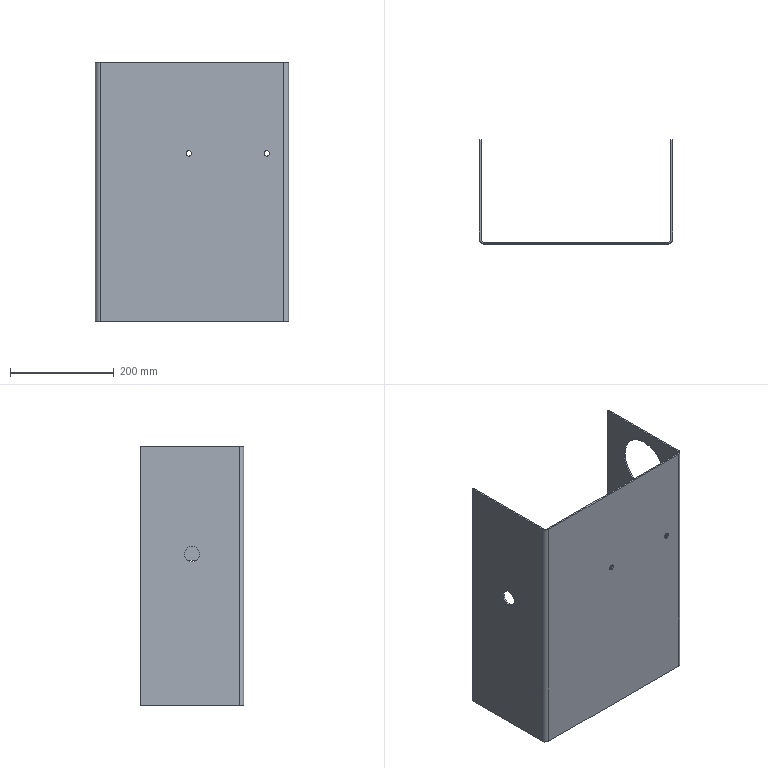Part | SolidWorks | features Cut 4, FlatPattern 1, SMBaseFlange 1, SheetMetal 1 | 1 solid | 34 faces | box 372 x 200 x 500 mm | volume 1068373 mm3 | plane 18 | cylinder 16 | commonest cylinder face diameters 10.5 x4 12 x2 18 x2 30 x2 50 x2 110 x2
STEP:
#1=CARTESIAN_POINT('',(-638.867,1083.196,324.485));
#2=VERTEX_POINT('',#1);
#3=CARTESIAN_POINT('',(-628.367,1083.196,324.485));
#4=VERTEX_POINT('',#3);
#5=CARTESIAN_POINT('',(-633.617,1083.196,324.485));
#6=DIRECTION('',(0.,-1.,0.));
#7=DIRECTION('',(1.,0.,0.));
#8=AXIS2_PLACEMENT_3D('',#5,#6,#7);
#9=CIRCLE('',#8,5.25);
#10=EDGE_CURVE('',#2,#4,#9,.T.);
#11=ORIENTED_EDGE('',*,*,#10,.F.);
#12=CARTESIAN_POINT('',(-638.867,1080.196,324.485));
#13=VERTEX_POINT('',#12);
#14=CARTESIAN_POINT('',(-638.867,1090.196,324.485));
#15=DIRECTION('',(0.,-1.,0.));
#16=VECTOR('',#15,1000.);
#17=LINE('',#14,#16);
#18=EDGE_CURVE('',#2,#13,#17,.T.);
#19=ORIENTED_EDGE('',*,*,#18,.T.);
#20=CARTESIAN_POINT('',(-628.367,1080.196,324.485));
#21=VERTEX_POINT('',#20);
#22=CARTESIAN_POINT('',(-633.617,1080.196,324.485));
#23=DIRECTION('',(0.,-1.,0.));
#24=DIRECTION('',(1.,0.,0.));
#25=AXIS2_PLACEMENT_3D('',#22,#23,#24);
#26=CIRCLE('',#25,5.25);
#27=EDGE_CURVE('',#13,#21,#26,.T.);
#28=ORIENTED_EDGE('',*,*,#27,.T.);
#29=CARTESIAN_POINT('',(-628.367,1090.196,324.485));
#30=DIRECTION('',(0.,-1.,0.));
#31=VECTOR('',#30,1000.);
#32=LINE('',#29,#31);
#33=EDGE_CURVE('',#4,#21,#32,.T.);
#34=ORIENTED_EDGE('',*,*,#33,.F.);
#35=EDGE_LOOP('',(#11,#19,#28,#34));
#36=FACE_OUTER_BOUND('',#35,.T.);
#37=CARTESIAN_POINT('',(-633.617,1090.196,324.485));
#38=DIRECTION('',(0.,-1.,0.));
#39=DIRECTION('',(1.,0.,0.));
#40=AXIS2_PLACEMENT_3D('',#37,#38,#39);
#41=CYLINDRICAL_SURFACE('',#40,5.25);
#42=ADVANCED_FACE('',(#36),#41,.F.);
#43=CARTESIAN_POINT('',(-788.867,1083.196,324.485));
#44=VERTEX_POINT('',#43);
#45=CARTESIAN_POINT('',(-778.367,1083.196,324.485));
#46=VERTEX_POINT('',#45);
#47=CARTESIAN_POINT('',(-783.617,1083.196,324.485));
#48=DIRECTION('',(0.,-1.,0.));
#49=DIRECTION('',(1.,0.,0.));
#50=AXIS2_PLACEMENT_3D('',#47,#48,#49);
#51=CIRCLE('',#50,5.25);
#52=EDGE_CURVE('',#44,#46,#51,.T.);
#53=ORIENTED_EDGE('',*,*,#52,.F.);
#54=CARTESIAN_POINT('',(-788.867,1080.196,324.485));
#55=VERTEX_POINT('',#54);
#56=CARTESIAN_POINT('',(-788.867,1090.196,324.485));
#57=DIRECTION('',(0.,-1.,0.));
#58=VECTOR('',#57,1000.);
#59=LINE('',#56,#58);
#60=EDGE_CURVE('',#44,#55,#59,.T.);
#61=ORIENTED_EDGE('',*,*,#60,.T.);
#62=CARTESIAN_POINT('',(-778.367,1080.196,324.485));
#63=VERTEX_POINT('',#62);
#64=CARTESIAN_POINT('',(-783.617,1080.196,324.485));
#65=DIRECTION('',(0.,-1.,0.));
#66=DIRECTION('',(1.,0.,0.));
#67=AXIS2_PLACEMENT_3D('',#64,#65,#66);
#68=CIRCLE('',#67,5.25);
#69=EDGE_CURVE('',#55,#63,#68,.T.);
#70=ORIENTED_EDGE('',*,*,#69,.T.);
#71=CARTESIAN_POINT('',(-778.367,1090.196,324.485));
#72=DIRECTION('',(0.,-1.,0.));
#73=VECTOR('',#72,1000.);
#74=LINE('',#71,#73);
#75=EDGE_CURVE('',#46,#63,#74,.T.);
#76=ORIENTED_EDGE('',*,*,#75,.F.);
#77=EDGE_LOOP('',(#53,#61,#70,#76));
#78=FACE_OUTER_BOUND('',#77,.T.);
#79=CARTESIAN_POINT('',(-783.617,1090.196,324.485));
#80=DIRECTION('',(0.,-1.,0.));
#81=DIRECTION('',(1.,0.,0.));
#82=AXIS2_PLACEMENT_3D('',#79,#80,#81);
#83=CYLINDRICAL_SURFACE('',#82,5.25);
#84=ADVANCED_FACE('',(#78),#83,.F.);
#85=CARTESIAN_POINT('',(-960.617,1195.196,292.));
#86=VERTEX_POINT('',#85);
#87=CARTESIAN_POINT('',(-960.617,1165.196,292.));
#88=VERTEX_POINT('',#87);
#89=CARTESIAN_POINT('',(-960.617,1180.196,292.));
#90=DIRECTION('',(-1.,0.,0.));
#91=DIRECTION('',(0.,-1.,0.));
#92=AXIS2_PLACEMENT_3D('',#89,#90,#91);
#93=CIRCLE('',#92,15.);
#94=EDGE_CURVE('',#86,#88,#93,.T.);
#95=ORIENTED_EDGE('',*,*,#94,.F.);
#96=CARTESIAN_POINT('',(-963.617,1195.196,292.));
#97=VERTEX_POINT('',#96);
#98=CARTESIAN_POINT('',(-953.617,1195.196,292.));
#99=DIRECTION('',(-1.,0.,0.));
#100=VECTOR('',#99,1000.);
#101=LINE('',#98,#100);
#102=EDGE_CURVE('',#86,#97,#101,.T.);
#103=ORIENTED_EDGE('',*,*,#102,.T.);
#104=CARTESIAN_POINT('',(-963.617,1165.196,292.));
#105=VERTEX_POINT('',#104);
#106=CARTESIAN_POINT('',(-963.617,1180.196,292.));
#107=DIRECTION('',(-1.,0.,0.));
#108=DIRECTION('',(0.,-1.,0.));
#109=AXIS2_PLACEMENT_3D('',#106,#107,#108);
#110=CIRCLE('',#109,15.);
#111=EDGE_CURVE('',#97,#105,#110,.T.);
#112=ORIENTED_EDGE('',*,*,#111,.T.);
#113=CARTESIAN_POINT('',(-953.617,1165.196,292.));
#114=DIRECTION('',(-1.,0.,0.));
#115=VECTOR('',#114,1000.);
#116=LINE('',#113,#115);
#117=EDGE_CURVE('',#88,#105,#116,.T.);
#118=ORIENTED_EDGE('',*,*,#117,.F.);
#119=EDGE_LOOP('',(#95,#103,#112,#118));
#120=FACE_OUTER_BOUND('',#119,.T.);
#121=CARTESIAN_POINT('',(-953.617,1180.196,292.));
#122=DIRECTION('',(-1.,0.,0.));
#123=DIRECTION('',(0.,-1.,0.));
#124=AXIS2_PLACEMENT_3D('',#121,#122,#123);
#125=CYLINDRICAL_SURFACE('',#124,15.);
#126=ADVANCED_FACE('',(#120),#125,.F.);
#127=CARTESIAN_POINT('',(-594.617,1137.696,95.));
#128=VERTEX_POINT('',#127);
#129=CARTESIAN_POINT('',(-594.617,1137.696,45.));
#130=VERTEX_POINT('',#129);
#131=CARTESIAN_POINT('',(-594.617,1137.696,70.));
#132=DIRECTION('',(1.,0.,0.));
#133=DIRECTION('',(0.,0.,-1.));
#134=AXIS2_PLACEMENT_3D('',#131,#132,#133);
#135=CIRCLE('',#134,25.);
#136=EDGE_CURVE('',#128,#130,#135,.T.);
#137=ORIENTED_EDGE('',*,*,#136,.F.);
#138=CARTESIAN_POINT('',(-591.617,1137.696,95.));
#139=VERTEX_POINT('',#138);
#140=CARTESIAN_POINT('',(-601.617,1137.696,95.));
#141=DIRECTION('',(1.,0.,0.));
#142=VECTOR('',#141,1000.);
#143=LINE('',#140,#142);
#144=EDGE_CURVE('',#128,#139,#143,.T.);
#145=ORIENTED_EDGE('',*,*,#144,.T.);
#146=CARTESIAN_POINT('',(-591.617,1137.696,45.));
#147=VERTEX_POINT('',#146);
#148=CARTESIAN_POINT('',(-591.617,1137.696,70.));
#149=DIRECTION('',(1.,0.,0.));
#150=DIRECTION('',(0.,0.,-1.));
#151=AXIS2_PLACEMENT_3D('',#148,#149,#150);
#152=CIRCLE('',#151,25.);
#153=EDGE_CURVE('',#139,#147,#152,.T.);
#154=ORIENTED_EDGE('',*,*,#153,.T.);
#155=CARTESIAN_POINT('',(-601.617,1137.696,45.));
#156=DIRECTION('',(1.,0.,0.));
#157=VECTOR('',#156,1000.);
#158=LINE('',#155,#157);
#159=EDGE_CURVE('',#130,#147,#158,.T.);
#160=ORIENTED_EDGE('',*,*,#159,.F.);
#161=EDGE_LOOP('',(#137,#145,#154,#160));
#162=FACE_OUTER_BOUND('',#161,.T.);
#163=CARTESIAN_POINT('',(-601.617,1137.696,70.));
#164=DIRECTION('',(1.,0.,0.));
#165=DIRECTION('',(0.,0.,-1.));
#166=AXIS2_PLACEMENT_3D('',#163,#164,#165);
#167=CYLINDRICAL_SURFACE('',#166,25.);
#168=ADVANCED_FACE('',(#162),#167,.F.);
#169=CARTESIAN_POINT('',(-594.617,1180.196,280.));
#170=VERTEX_POINT('',#169);
#171=CARTESIAN_POINT('',(-594.617,1180.196,160.));
#172=VERTEX_POINT('',#171);
#173=CARTESIAN_POINT('',(-594.617,1180.196,220.));
#174=DIRECTION('',(1.,0.,0.));
#175=DIRECTION('',(0.,0.,-1.));
#176=AXIS2_PLACEMENT_3D('',#173,#174,#175);
#177=CIRCLE('',#176,60.);
#178=EDGE_CURVE('',#170,#172,#177,.T.);
#179=ORIENTED_EDGE('',*,*,#178,.F.);
#180=CARTESIAN_POINT('',(-591.617,1180.196,280.));
#181=VERTEX_POINT('',#180);
#182=CARTESIAN_POINT('',(-601.617,1180.196,280.));
#183=DIRECTION('',(1.,0.,0.));
#184=VECTOR('',#183,1000.);
#185=LINE('',#182,#184);
#186=EDGE_CURVE('',#170,#181,#185,.T.);
#187=ORIENTED_EDGE('',*,*,#186,.T.);
#188=CARTESIAN_POINT('',(-591.617,1180.196,160.));
#189=VERTEX_POINT('',#188);
#190=CARTESIAN_POINT('',(-591.617,1180.196,220.));
#191=DIRECTION('',(1.,0.,0.));
#192=DIRECTION('',(0.,0.,-1.));
#193=AXIS2_PLACEMENT_3D('',#190,#191,#192);
#194=CIRCLE('',#193,60.);
#195=EDGE_CURVE('',#181,#189,#194,.T.);
#196=ORIENTED_EDGE('',*,*,#195,.T.);
#197=CARTESIAN_POINT('',(-601.617,1180.196,160.));
#198=DIRECTION('',(1.,0.,0.));
#199=VECTOR('',#198,1000.);
#200=LINE('',#197,#199);
#201=EDGE_CURVE('',#172,#189,#200,.T.);
#202=ORIENTED_EDGE('',*,*,#201,.F.);
#203=EDGE_LOOP('',(#179,#187,#196,#202));
#204=FACE_OUTER_BOUND('',#203,.T.);
#205=CARTESIAN_POINT('',(-601.617,1180.196,220.));
#206=DIRECTION('',(1.,0.,0.));
#207=DIRECTION('',(0.,0.,-1.));
#208=AXIS2_PLACEMENT_3D('',#205,#206,#207);
#209=CYLINDRICAL_SURFACE('',#208,60.);
#210=ADVANCED_FACE('',(#204),#209,.F.);
#211=CARTESIAN_POINT('',(-594.617,1180.196,475.));
#212=VERTEX_POINT('',#211);
#213=CARTESIAN_POINT('',(-594.617,1180.196,365.));
#214=VERTEX_POINT('',#213);
#215=CARTESIAN_POINT('',(-594.617,1180.196,420.));
#216=DIRECTION('',(1.,0.,0.));
#217=DIRECTION('',(0.,0.,-1.));
#218=AXIS2_PLACEMENT_3D('',#215,#216,#217);
#219=CIRCLE('',#218,55.);
#220=EDGE_CURVE('',#212,#214,#219,.T.);
#221=ORIENTED_EDGE('',*,*,#220,.F.);
#222=CARTESIAN_POINT('',(-591.617,1180.196,475.));
#223=VERTEX_POINT('',#222);
#224=CARTESIAN_POINT('',(-601.617,1180.196,475.));
#225=DIRECTION('',(1.,0.,0.));
#226=VECTOR('',#225,1000.);
#227=LINE('',#224,#226);
#228=EDGE_CURVE('',#212,#223,#227,.T.);
#229=ORIENTED_EDGE('',*,*,#228,.T.);
#230=CARTESIAN_POINT('',(-591.617,1180.196,365.));
#231=VERTEX_POINT('',#230);
#232=CARTESIAN_POINT('',(-591.617,1180.196,420.));
#233=DIRECTION('',(1.,0.,0.));
#234=DIRECTION('',(0.,0.,-1.));
#235=AXIS2_PLACEMENT_3D('',#232,#233,#234);
#236=CIRCLE('',#235,55.);
#237=EDGE_CURVE('',#223,#231,#236,.T.);
#238=ORIENTED_EDGE('',*,*,#237,.T.);
#239=CARTESIAN_POINT('',(-601.617,1180.196,365.));
#240=DIRECTION('',(1.,0.,0.));
#241=VECTOR('',#240,1000.);
#242=LINE('',#239,#241);
#243=EDGE_CURVE('',#214,#231,#242,.T.);
#244=ORIENTED_EDGE('',*,*,#243,.F.);
#245=EDGE_LOOP('',(#221,#229,#238,#244));
#246=FACE_OUTER_BOUND('',#245,.T.);
#247=CARTESIAN_POINT('',(-601.617,1180.196,420.));
#248=DIRECTION('',(1.,0.,0.));
#249=DIRECTION('',(0.,0.,-1.));
#250=AXIS2_PLACEMENT_3D('',#247,#248,#249);
#251=CYLINDRICAL_SURFACE('',#250,55.);
#252=ADVANCED_FACE('',(#246),#251,.F.);
#253=CARTESIAN_POINT('',(-600.617,1080.196,500.));
#254=VERTEX_POINT('',#253);
#255=CARTESIAN_POINT('',(-600.617,1083.196,500.));
#256=VERTEX_POINT('',#255);
#257=CARTESIAN_POINT('',(-600.617,1080.196,500.));
#258=DIRECTION('',(0.,1.,0.));
#259=VECTOR('',#258,1000.);
#260=LINE('',#257,#259);
#261=EDGE_CURVE('',#254,#256,#260,.T.);
#262=ORIENTED_EDGE('',*,*,#261,.F.);
#263=CARTESIAN_POINT('',(-591.617,1089.196,500.));
#264=VERTEX_POINT('',#263);
#265=CARTESIAN_POINT('',(-600.617,1089.196,500.));
#266=DIRECTION('',(0.,0.,-1.));
#267=DIRECTION('',(1.,0.,0.));
#268=AXIS2_PLACEMENT_3D('',#265,#266,#267);
#269=CIRCLE('',#268,9.);
#270=EDGE_CURVE('',#264,#254,#269,.T.);
#271=ORIENTED_EDGE('',*,*,#270,.F.);
#272=CARTESIAN_POINT('',(-594.617,1089.196,500.));
#273=VERTEX_POINT('',#272);
#274=CARTESIAN_POINT('',(-594.617,1089.196,500.));
#275=DIRECTION('',(1.,0.,0.));
#276=VECTOR('',#275,1000.);
#277=LINE('',#274,#276);
#278=EDGE_CURVE('',#273,#264,#277,.T.);
#279=ORIENTED_EDGE('',*,*,#278,.F.);
#280=CARTESIAN_POINT('',(-600.617,1089.196,500.));
#281=DIRECTION('',(0.,0.,-1.));
#282=DIRECTION('',(1.,0.,0.));
#283=AXIS2_PLACEMENT_3D('',#280,#281,#282);
#284=CIRCLE('',#283,6.);
#285=EDGE_CURVE('',#273,#256,#284,.T.);
#286=ORIENTED_EDGE('',*,*,#285,.T.);
#287=EDGE_LOOP('',(#262,#271,#279,#286));
#288=FACE_OUTER_BOUND('',#287,.T.);
#289=CARTESIAN_POINT('',(-600.617,1080.196,500.));
#290=DIRECTION('',(0.,0.,1.));
#291=DIRECTION('',(1.,0.,0.));
#292=AXIS2_PLACEMENT_3D('',#289,#290,#291);
#293=PLANE('',#292);
#294=ADVANCED_FACE('',(#288),#293,.T.);
#295=CARTESIAN_POINT('',(-954.617,1080.196,500.));
#296=VERTEX_POINT('',#295);
#297=CARTESIAN_POINT('',(-954.617,1080.196,500.));
#298=DIRECTION('',(-1.,0.,0.));
#299=VECTOR('',#298,1000.);
#300=LINE('',#297,#299);
#301=EDGE_CURVE('',#254,#296,#300,.T.);
#302=ORIENTED_EDGE('',*,*,#301,.F.);
#303=ORIENTED_EDGE('',*,*,#261,.T.);
#304=CARTESIAN_POINT('',(-954.617,1083.196,500.));
#305=VERTEX_POINT('',#304);
#306=CARTESIAN_POINT('',(-954.617,1083.196,500.));
#307=DIRECTION('',(-1.,0.,0.));
#308=VECTOR('',#307,1000.);
#309=LINE('',#306,#308);
#310=EDGE_CURVE('',#256,#305,#309,.T.);
#311=ORIENTED_EDGE('',*,*,#310,.T.);
#312=CARTESIAN_POINT('',(-954.617,1083.196,500.));
#313=DIRECTION('',(0.,-1.,0.));
#314=VECTOR('',#313,1000.);
#315=LINE('',#312,#314);
#316=EDGE_CURVE('',#305,#296,#315,.T.);
#317=ORIENTED_EDGE('',*,*,#316,.T.);
#318=EDGE_LOOP('',(#302,#303,#311,#317));
#319=FACE_OUTER_BOUND('',#318,.T.);
#320=CARTESIAN_POINT('',(-594.617,1089.196,500.));
#321=DIRECTION('',(0.,0.,1.));
#322=DIRECTION('',(1.,0.,0.));
#323=AXIS2_PLACEMENT_3D('',#320,#321,#322);
#324=PLANE('',#323);
#325=ADVANCED_FACE('',(#319),#324,.T.);
#326=CARTESIAN_POINT('',(-591.617,1089.196,0.));
#327=VERTEX_POINT('',#326);
#328=CARTESIAN_POINT('',(-594.617,1089.196,0.));
#329=VERTEX_POINT('',#328);
#330=CARTESIAN_POINT('',(-591.617,1089.196,0.));
#331=DIRECTION('',(-1.,0.,0.));
#332=VECTOR('',#331,1000.);
#333=LINE('',#330,#332);
#334=EDGE_CURVE('',#327,#329,#333,.T.);
#335=ORIENTED_EDGE('',*,*,#334,.F.);
#336=CARTESIAN_POINT('',(-600.617,1080.196,0.));
#337=VERTEX_POINT('',#336);
#338=CARTESIAN_POINT('',(-600.617,1089.196,0.));
#339=DIRECTION('',(0.,0.,-1.));
#340=DIRECTION('',(1.,0.,0.));
#341=AXIS2_PLACEMENT_3D('',#338,#339,#340);
#342=CIRCLE('',#341,9.);
#343=EDGE_CURVE('',#327,#337,#342,.T.);
#344=ORIENTED_EDGE('',*,*,#343,.T.);
#345=CARTESIAN_POINT('',(-600.617,1083.196,0.));
#346=VERTEX_POINT('',#345);
#347=CARTESIAN_POINT('',(-600.617,1083.196,0.));
#348=DIRECTION('',(0.,-1.,0.));
#349=VECTOR('',#348,1000.);
#350=LINE('',#347,#349);
#351=EDGE_CURVE('',#346,#337,#350,.T.);
#352=ORIENTED_EDGE('',*,*,#351,.F.);
#353=CARTESIAN_POINT('',(-600.617,1089.196,0.));
#354=DIRECTION('',(0.,0.,-1.));
#355=DIRECTION('',(1.,0.,0.));
#356=AXIS2_PLACEMENT_3D('',#353,#354,#355);
#357=CIRCLE('',#356,6.);
#358=EDGE_CURVE('',#329,#346,#357,.T.);
#359=ORIENTED_EDGE('',*,*,#358,.F.);
#360=EDGE_LOOP('',(#335,#344,#352,#359));
#361=FACE_OUTER_BOUND('',#360,.T.);
#362=CARTESIAN_POINT('',(-591.617,1089.196,0.));
#363=DIRECTION('',(0.,0.,-1.));
#364=DIRECTION('',(-1.,0.,0.));
#365=AXIS2_PLACEMENT_3D('',#362,#363,#364);
#366=PLANE('',#365);
#367=ADVANCED_FACE('',(#361),#366,.T.);
#368=CARTESIAN_POINT('',(-591.617,1280.196,0.));
#369=VERTEX_POINT('',#368);
#370=CARTESIAN_POINT('',(-591.617,1089.196,0.));
#371=DIRECTION('',(0.,-1.,0.));
#372=VECTOR('',#371,1000.);
#373=LINE('',#370,#372);
#374=EDGE_CURVE('',#369,#327,#373,.T.);
#375=ORIENTED_EDGE('',*,*,#374,.T.);
#376=ORIENTED_EDGE('',*,*,#334,.T.);
#377=CARTESIAN_POINT('',(-594.617,1280.196,0.));
#378=VERTEX_POINT('',#377);
#379=CARTESIAN_POINT('',(-594.617,1089.196,0.));
#380=DIRECTION('',(0.,-1.,0.));
#381=VECTOR('',#380,1000.);
#382=LINE('',#379,#381);
#383=EDGE_CURVE('',#378,#329,#382,.T.);
#384=ORIENTED_EDGE('',*,*,#383,.F.);
#385=CARTESIAN_POINT('',(-594.617,1280.196,0.));
#386=DIRECTION('',(1.,0.,0.));
#387=VECTOR('',#386,1000.);
#388=LINE('',#385,#387);
#389=EDGE_CURVE('',#378,#369,#388,.T.);
#390=ORIENTED_EDGE('',*,*,#389,.T.);
#391=EDGE_LOOP('',(#375,#376,#384,#390));
#392=FACE_OUTER_BOUND('',#391,.T.);
#393=CARTESIAN_POINT('',(-600.617,1083.196,0.));
#394=DIRECTION('',(0.,0.,-1.));
#395=DIRECTION('',(-1.,0.,0.));
#396=AXIS2_PLACEMENT_3D('',#393,#394,#395);
#397=PLANE('',#396);
#398=ADVANCED_FACE('',(#392),#397,.T.);
#399=CARTESIAN_POINT('',(-963.617,1089.196,500.));
#400=VERTEX_POINT('',#399);
#401=CARTESIAN_POINT('',(-960.617,1089.196,500.));
#402=VERTEX_POINT('',#401);
#403=CARTESIAN_POINT('',(-963.617,1089.196,500.));
#404=DIRECTION('',(1.,0.,0.));
#405=VECTOR('',#404,1000.);
#406=LINE('',#403,#405);
#407=EDGE_CURVE('',#400,#402,#406,.T.);
#408=ORIENTED_EDGE('',*,*,#407,.F.);
#409=CARTESIAN_POINT('',(-954.617,1089.196,500.));
#410=DIRECTION('',(0.,0.,-1.));
#411=DIRECTION('',(1.,0.,0.));
#412=AXIS2_PLACEMENT_3D('',#409,#410,#411);
#413=CIRCLE('',#412,9.);
#414=EDGE_CURVE('',#296,#400,#413,.T.);
#415=ORIENTED_EDGE('',*,*,#414,.F.);
#416=ORIENTED_EDGE('',*,*,#316,.F.);
#417=CARTESIAN_POINT('',(-954.617,1089.196,500.));
#418=DIRECTION('',(0.,0.,-1.));
#419=DIRECTION('',(1.,0.,0.));
#420=AXIS2_PLACEMENT_3D('',#417,#418,#419);
#421=CIRCLE('',#420,6.);
#422=EDGE_CURVE('',#305,#402,#421,.T.);
#423=ORIENTED_EDGE('',*,*,#422,.T.);
#424=EDGE_LOOP('',(#408,#415,#416,#423));
#425=FACE_OUTER_BOUND('',#424,.T.);
#426=CARTESIAN_POINT('',(-963.617,1089.196,500.));
#427=DIRECTION('',(0.,0.,1.));
#428=DIRECTION('',(1.,0.,0.));
#429=AXIS2_PLACEMENT_3D('',#426,#427,#428);
#430=PLANE('',#429);
#431=ADVANCED_FACE('',(#425),#430,.T.);
#432=CARTESIAN_POINT('',(-963.617,1280.196,500.));
#433=VERTEX_POINT('',#432);
#434=CARTESIAN_POINT('',(-963.617,1089.196,500.));
#435=DIRECTION('',(0.,1.,0.));
#436=VECTOR('',#435,1000.);
#437=LINE('',#434,#436);
#438=EDGE_CURVE('',#400,#433,#437,.T.);
#439=ORIENTED_EDGE('',*,*,#438,.F.);
#440=ORIENTED_EDGE('',*,*,#407,.T.);
#441=CARTESIAN_POINT('',(-960.617,1280.196,500.));
#442=VERTEX_POINT('',#441);
#443=CARTESIAN_POINT('',(-960.617,1089.196,500.));
#444=DIRECTION('',(0.,1.,0.));
#445=VECTOR('',#444,1000.);
#446=LINE('',#443,#445);
#447=EDGE_CURVE('',#402,#442,#446,.T.);
#448=ORIENTED_EDGE('',*,*,#447,.T.);
#449=CARTESIAN_POINT('',(-963.617,1280.196,500.));
#450=DIRECTION('',(1.,0.,0.));
#451=VECTOR('',#450,1000.);
#452=LINE('',#449,#451);
#453=EDGE_CURVE('',#433,#442,#452,.T.);
#454=ORIENTED_EDGE('',*,*,#453,.F.);
#455=EDGE_LOOP('',(#439,#440,#448,#454));
#456=FACE_OUTER_BOUND('',#455,.T.);
#457=CARTESIAN_POINT('',(-954.617,1083.196,500.));
#458=DIRECTION('',(0.,0.,1.));
#459=DIRECTION('',(1.,0.,0.));
#460=AXIS2_PLACEMENT_3D('',#457,#458,#459);
#461=PLANE('',#460);
#462=ADVANCED_FACE('',(#456),#461,.T.);
#463=CARTESIAN_POINT('',(-954.617,1080.196,0.));
#464=VERTEX_POINT('',#463);
#465=CARTESIAN_POINT('',(-954.617,1083.196,0.));
#466=VERTEX_POINT('',#465);
#467=CARTESIAN_POINT('',(-954.617,1080.196,0.));
#468=DIRECTION('',(0.,1.,0.));
#469=VECTOR('',#468,1000.);
#470=LINE('',#467,#469);
#471=EDGE_CURVE('',#464,#466,#470,.T.);
#472=ORIENTED_EDGE('',*,*,#471,.F.);
#473=CARTESIAN_POINT('',(-963.617,1089.196,0.));
#474=VERTEX_POINT('',#473);
#475=CARTESIAN_POINT('',(-954.617,1089.196,0.));
#476=DIRECTION('',(0.,0.,-1.));
#477=DIRECTION('',(1.,0.,0.));
#478=AXIS2_PLACEMENT_3D('',#475,#476,#477);
#479=CIRCLE('',#478,9.);
#480=EDGE_CURVE('',#464,#474,#479,.T.);
#481=ORIENTED_EDGE('',*,*,#480,.T.);
#482=CARTESIAN_POINT('',(-960.617,1089.196,0.));
#483=VERTEX_POINT('',#482);
#484=CARTESIAN_POINT('',(-960.617,1089.196,0.));
#485=DIRECTION('',(-1.,0.,0.));
#486=VECTOR('',#485,1000.);
#487=LINE('',#484,#486);
#488=EDGE_CURVE('',#483,#474,#487,.T.);
#489=ORIENTED_EDGE('',*,*,#488,.F.);
#490=CARTESIAN_POINT('',(-954.617,1089.196,0.));
#491=DIRECTION('',(0.,0.,-1.));
#492=DIRECTION('',(1.,0.,0.));
#493=AXIS2_PLACEMENT_3D('',#490,#491,#492);
#494=CIRCLE('',#493,6.);
#495=EDGE_CURVE('',#466,#483,#494,.T.);
#496=ORIENTED_EDGE('',*,*,#495,.F.);
#497=EDGE_LOOP('',(#472,#481,#489,#496));
#498=FACE_OUTER_BOUND('',#497,.T.);
#499=CARTESIAN_POINT('',(-954.617,1080.196,0.));
#500=DIRECTION('',(0.,0.,-1.));
#501=DIRECTION('',(-1.,0.,0.));
#502=AXIS2_PLACEMENT_3D('',#499,#500,#501);
#503=PLANE('',#502);
#504=ADVANCED_FACE('',(#498),#503,.T.);
#505=CARTESIAN_POINT('',(-954.617,1080.196,0.));
#506=DIRECTION('',(-1.,0.,0.));
#507=VECTOR('',#506,1000.);
#508=LINE('',#505,#507);
#509=EDGE_CURVE('',#337,#464,#508,.T.);
#510=ORIENTED_EDGE('',*,*,#509,.T.);
#511=ORIENTED_EDGE('',*,*,#471,.T.);
#512=CARTESIAN_POINT('',(-954.617,1083.196,0.));
#513=DIRECTION('',(-1.,0.,0.));
#514=VECTOR('',#513,1000.);
#515=LINE('',#512,#514);
#516=EDGE_CURVE('',#346,#466,#515,.T.);
#517=ORIENTED_EDGE('',*,*,#516,.F.);
#518=ORIENTED_EDGE('',*,*,#351,.T.);
#519=EDGE_LOOP('',(#510,#511,#517,#518));
#520=FACE_OUTER_BOUND('',#519,.T.);
#521=CARTESIAN_POINT('',(-960.617,1089.196,0.));
#522=DIRECTION('',(0.,0.,-1.));
#523=DIRECTION('',(-1.,0.,0.));
#524=AXIS2_PLACEMENT_3D('',#521,#522,#523);
#525=PLANE('',#524);
#526=ADVANCED_FACE('',(#520),#525,.T.);
#527=CARTESIAN_POINT('',(-960.617,1180.196,292.));
#528=DIRECTION('',(-1.,0.,0.));
#529=DIRECTION('',(0.,-1.,0.));
#530=AXIS2_PLACEMENT_3D('',#527,#528,#529);
#531=CIRCLE('',#530,15.);
#532=EDGE_CURVE('',#88,#86,#531,.T.);
#533=ORIENTED_EDGE('',*,*,#532,.T.);
#534=ORIENTED_EDGE('',*,*,#94,.T.);
#535=EDGE_LOOP('',(#533,#534));
#536=FACE_BOUND('',#535,.T.);
#537=CARTESIAN_POINT('',(-960.617,1280.196,0.));
#538=VERTEX_POINT('',#537);
#539=CARTESIAN_POINT('',(-960.617,1089.196,0.));
#540=DIRECTION('',(0.,1.,0.));
#541=VECTOR('',#540,1000.);
#542=LINE('',#539,#541);
#543=EDGE_CURVE('',#483,#538,#542,.T.);
#544=ORIENTED_EDGE('',*,*,#543,.T.);
#545=CARTESIAN_POINT('',(-960.617,1280.196,500.));
#546=DIRECTION('',(0.,0.,-1.));
#547=VECTOR('',#546,1000.);
#548=LINE('',#545,#547);
#549=EDGE_CURVE('',#442,#538,#548,.T.);
#550=ORIENTED_EDGE('',*,*,#549,.F.);
#551=ORIENTED_EDGE('',*,*,#447,.F.);
#552=CARTESIAN_POINT('',(-960.617,1089.196,500.));
#553=DIRECTION('',(0.,0.,-1.));
#554=VECTOR('',#553,1000.);
#555=LINE('',#552,#554);
#556=EDGE_CURVE('',#402,#483,#555,.T.);
#557=ORIENTED_EDGE('',*,*,#556,.T.);
#558=EDGE_LOOP('',(#544,#550,#551,#557));
#559=FACE_OUTER_BOUND('',#558,.T.);
#560=CARTESIAN_POINT('',(-960.617,1089.196,500.));
#561=DIRECTION('',(-1.,0.,0.));
#562=DIRECTION('',(0.,-1.,0.));
#563=AXIS2_PLACEMENT_3D('',#560,#561,#562);
#564=PLANE('',#563);
#565=ADVANCED_FACE('',(#536,#559),#564,.F.);
#566=CARTESIAN_POINT('',(-963.617,1280.196,0.));
#567=VERTEX_POINT('',#566);
#568=CARTESIAN_POINT('',(-963.617,1280.196,0.));
#569=DIRECTION('',(1.,0.,0.));
#570=VECTOR('',#569,1000.);
#571=LINE('',#568,#570);
#572=EDGE_CURVE('',#567,#538,#571,.T.);
#573=ORIENTED_EDGE('',*,*,#572,.F.);
#574=CARTESIAN_POINT('',(-963.617,1280.196,500.));
#575=DIRECTION('',(0.,0.,-1.));
#576=VECTOR('',#575,1000.);
#577=LINE('',#574,#576);
#578=EDGE_CURVE('',#433,#567,#577,.T.);
#579=ORIENTED_EDGE('',*,*,#578,.F.);
#580=ORIENTED_EDGE('',*,*,#453,.T.);
#581=ORIENTED_EDGE('',*,*,#549,.T.);
#582=EDGE_LOOP('',(#573,#579,#580,#581));
#583=FACE_OUTER_BOUND('',#582,.T.);
#584=CARTESIAN_POINT('',(-963.617,1280.196,500.));
#585=DIRECTION('',(0.,1.,0.));
#586=DIRECTION('',(0.,0.,1.));
#587=AXIS2_PLACEMENT_3D('',#584,#585,#586);
#588=PLANE('',#587);
#589=ADVANCED_FACE('',(#583),#588,.T.);
#590=CARTESIAN_POINT('',(-963.617,1180.196,292.));
#591=DIRECTION('',(-1.,0.,0.));
#592=DIRECTION('',(0.,-1.,0.));
#593=AXIS2_PLACEMENT_3D('',#590,#591,#592);
#594=CIRCLE('',#593,15.);
#595=EDGE_CURVE('',#105,#97,#594,.T.);
#596=ORIENTED_EDGE('',*,*,#595,.F.);
#597=ORIENTED_EDGE('',*,*,#111,.F.);
#598=EDGE_LOOP('',(#596,#597));
#599=FACE_BOUND('',#598,.T.);
#600=CARTESIAN_POINT('',(-963.617,1089.196,0.));
#601=DIRECTION('',(0.,1.,0.));
#602=VECTOR('',#601,1000.);
#603=LINE('',#600,#602);
#604=EDGE_CURVE('',#474,#567,#603,.T.);
#605=ORIENTED_EDGE('',*,*,#604,.F.);
#606=CARTESIAN_POINT('',(-963.617,1089.196,500.));
#607=DIRECTION('',(0.,0.,-1.));
#608=VECTOR('',#607,1000.);
#609=LINE('',#606,#608);
#610=EDGE_CURVE('',#400,#474,#609,.T.);
#611=ORIENTED_EDGE('',*,*,#610,.F.);
#612=ORIENTED_EDGE('',*,*,#438,.T.);
#613=ORIENTED_EDGE('',*,*,#578,.T.);
#614=EDGE_LOOP('',(#605,#611,#612,#613));
#615=FACE_OUTER_BOUND('',#614,.T.);
#616=CARTESIAN_POINT('',(-963.617,1089.196,500.));
#617=DIRECTION('',(-1.,0.,0.));
#618=DIRECTION('',(0.,-1.,0.));
#619=AXIS2_PLACEMENT_3D('',#616,#617,#618);
#620=PLANE('',#619);
#621=ADVANCED_FACE('',(#599,#615),#620,.T.);
#622=ORIENTED_EDGE('',*,*,#480,.F.);
#623=CARTESIAN_POINT('',(-954.617,1080.196,500.));
#624=DIRECTION('',(0.,0.,-1.));
#625=VECTOR('',#624,1000.);
#626=LINE('',#623,#625);
#627=EDGE_CURVE('',#296,#464,#626,.T.);
#628=ORIENTED_EDGE('',*,*,#627,.F.);
#629=ORIENTED_EDGE('',*,*,#414,.T.);
#630=ORIENTED_EDGE('',*,*,#610,.T.);
#631=EDGE_LOOP('',(#622,#628,#629,#630));
#632=FACE_OUTER_BOUND('',#631,.T.);
#633=CARTESIAN_POINT('',(-954.617,1089.196,500.));
#634=DIRECTION('',(0.,0.,-1.));
#635=DIRECTION('',(-1.,0.,0.));
#636=AXIS2_PLACEMENT_3D('',#633,#634,#635);
#637=CYLINDRICAL_SURFACE('',#636,9.);
#638=ADVANCED_FACE('',(#632),#637,.T.);
#639=CARTESIAN_POINT('',(-633.617,1080.196,324.485));
#640=DIRECTION('',(0.,-1.,0.));
#641=DIRECTION('',(1.,0.,0.));
#642=AXIS2_PLACEMENT_3D('',#639,#640,#641);
#643=CIRCLE('',#642,5.25);
#644=EDGE_CURVE('',#21,#13,#643,.T.);
#645=ORIENTED_EDGE('',*,*,#644,.F.);
#646=ORIENTED_EDGE('',*,*,#27,.F.);
#647=EDGE_LOOP('',(#645,#646));
#648=FACE_BOUND('',#647,.T.);
#649=CARTESIAN_POINT('',(-783.617,1080.196,324.485));
#650=DIRECTION('',(0.,-1.,0.));
#651=DIRECTION('',(1.,0.,0.));
#652=AXIS2_PLACEMENT_3D('',#649,#650,#651);
#653=CIRCLE('',#652,5.25);
#654=EDGE_CURVE('',#63,#55,#653,.T.);
#655=ORIENTED_EDGE('',*,*,#654,.F.);
#656=ORIENTED_EDGE('',*,*,#69,.F.);
#657=EDGE_LOOP('',(#655,#656));
#658=FACE_BOUND('',#657,.T.);
#659=ORIENTED_EDGE('',*,*,#509,.F.);
#660=CARTESIAN_POINT('',(-600.617,1080.196,500.));
#661=DIRECTION('',(0.,0.,-1.));
#662=VECTOR('',#661,1000.);
#663=LINE('',#660,#662);
#664=EDGE_CURVE('',#254,#337,#663,.T.);
#665=ORIENTED_EDGE('',*,*,#664,.F.);
#666=ORIENTED_EDGE('',*,*,#301,.T.);
#667=ORIENTED_EDGE('',*,*,#627,.T.);
#668=EDGE_LOOP('',(#659,#665,#666,#667));
#669=FACE_OUTER_BOUND('',#668,.T.);
#670=CARTESIAN_POINT('',(-954.617,1080.196,500.));
#671=DIRECTION('',(0.,-1.,0.));
#672=DIRECTION('',(1.,0.,0.));
#673=AXIS2_PLACEMENT_3D('',#670,#671,#672);
#674=PLANE('',#673);
#675=ADVANCED_FACE('',(#648,#658,#669),#674,.T.);
#676=ORIENTED_EDGE('',*,*,#343,.F.);
#677=CARTESIAN_POINT('',(-591.617,1089.196,500.));
#678=DIRECTION('',(0.,0.,-1.));
#679=VECTOR('',#678,1000.);
#680=LINE('',#677,#679);
#681=EDGE_CURVE('',#264,#327,#680,.T.);
#682=ORIENTED_EDGE('',*,*,#681,.F.);
#683=ORIENTED_EDGE('',*,*,#270,.T.);
#684=ORIENTED_EDGE('',*,*,#664,.T.);
#685=EDGE_LOOP('',(#676,#682,#683,#684));
#686=FACE_OUTER_BOUND('',#685,.T.);
#687=CARTESIAN_POINT('',(-600.617,1089.196,500.));
#688=DIRECTION('',(0.,0.,-1.));
#689=DIRECTION('',(-1.,0.,0.));
#690=AXIS2_PLACEMENT_3D('',#687,#688,#689);
#691=CYLINDRICAL_SURFACE('',#690,9.);
#692=ADVANCED_FACE('',(#686),#691,.T.);
#693=CARTESIAN_POINT('',(-591.617,1137.696,70.));
#694=DIRECTION('',(1.,0.,0.));
#695=DIRECTION('',(0.,0.,-1.));
#696=AXIS2_PLACEMENT_3D('',#693,#694,#695);
#697=CIRCLE('',#696,25.);
#698=EDGE_CURVE('',#147,#139,#697,.T.);
#699=ORIENTED_EDGE('',*,*,#698,.F.);
#700=ORIENTED_EDGE('',*,*,#153,.F.);
#701=EDGE_LOOP('',(#699,#700));
#702=FACE_BOUND('',#701,.T.);
#703=CARTESIAN_POINT('',(-591.617,1180.196,220.));
#704=DIRECTION('',(1.,0.,0.));
#705=DIRECTION('',(0.,0.,-1.));
#706=AXIS2_PLACEMENT_3D('',#703,#704,#705);
#707=CIRCLE('',#706,60.);
#708=EDGE_CURVE('',#189,#181,#707,.T.);
#709=ORIENTED_EDGE('',*,*,#708,.F.);
#710=ORIENTED_EDGE('',*,*,#195,.F.);
#711=EDGE_LOOP('',(#709,#710));
#712=FACE_BOUND('',#711,.T.);
#713=CARTESIAN_POINT('',(-591.617,1180.196,420.));
#714=DIRECTION('',(1.,0.,0.));
#715=DIRECTION('',(0.,0.,-1.));
#716=AXIS2_PLACEMENT_3D('',#713,#714,#715);
#717=CIRCLE('',#716,55.);
#718=EDGE_CURVE('',#231,#223,#717,.T.);
#719=ORIENTED_EDGE('',*,*,#718,.F.);
#720=ORIENTED_EDGE('',*,*,#237,.F.);
#721=EDGE_LOOP('',(#719,#720));
#722=FACE_BOUND('',#721,.T.);
#723=ORIENTED_EDGE('',*,*,#374,.F.);
#724=CARTESIAN_POINT('',(-591.617,1280.196,500.));
#725=VERTEX_POINT('',#724);
#726=CARTESIAN_POINT('',(-591.617,1280.196,500.));
#727=DIRECTION('',(0.,0.,-1.));
#728=VECTOR('',#727,1000.);
#729=LINE('',#726,#728);
#730=EDGE_CURVE('',#725,#369,#729,.T.);
#731=ORIENTED_EDGE('',*,*,#730,.F.);
#732=CARTESIAN_POINT('',(-591.617,1089.196,500.));
#733=DIRECTION('',(0.,-1.,0.));
#734=VECTOR('',#733,1000.);
#735=LINE('',#732,#734);
#736=EDGE_CURVE('',#725,#264,#735,.T.);
#737=ORIENTED_EDGE('',*,*,#736,.T.);
#738=ORIENTED_EDGE('',*,*,#681,.T.);
#739=EDGE_LOOP('',(#723,#731,#737,#738));
#740=FACE_OUTER_BOUND('',#739,.T.);
#741=CARTESIAN_POINT('',(-591.617,1089.196,500.));
#742=DIRECTION('',(1.,0.,0.));
#743=DIRECTION('',(0.,0.,-1.));
#744=AXIS2_PLACEMENT_3D('',#741,#742,#743);
#745=PLANE('',#744);
#746=ADVANCED_FACE('',(#702,#712,#722,#740),#745,.T.);
#747=ORIENTED_EDGE('',*,*,#389,.F.);
#748=CARTESIAN_POINT('',(-594.617,1280.196,500.));
#749=VERTEX_POINT('',#748);
#750=CARTESIAN_POINT('',(-594.617,1280.196,500.));
#751=DIRECTION('',(0.,0.,-1.));
#752=VECTOR('',#751,1000.);
#753=LINE('',#750,#752);
#754=EDGE_CURVE('',#749,#378,#753,.T.);
#755=ORIENTED_EDGE('',*,*,#754,.F.);
#756=CARTESIAN_POINT('',(-594.617,1280.196,500.));
#757=DIRECTION('',(1.,0.,0.));
#758=VECTOR('',#757,1000.);
#759=LINE('',#756,#758);
#760=EDGE_CURVE('',#749,#725,#759,.T.);
#761=ORIENTED_EDGE('',*,*,#760,.T.);
#762=ORIENTED_EDGE('',*,*,#730,.T.);
#763=EDGE_LOOP('',(#747,#755,#761,#762));
#764=FACE_OUTER_BOUND('',#763,.T.);
#765=CARTESIAN_POINT('',(-594.617,1280.196,500.));
#766=DIRECTION('',(0.,1.,0.));
#767=DIRECTION('',(0.,0.,1.));
#768=AXIS2_PLACEMENT_3D('',#765,#766,#767);
#769=PLANE('',#768);
#770=ADVANCED_FACE('',(#764),#769,.T.);
#771=CARTESIAN_POINT('',(-594.617,1137.696,70.));
#772=DIRECTION('',(1.,0.,0.));
#773=DIRECTION('',(0.,0.,-1.));
#774=AXIS2_PLACEMENT_3D('',#771,#772,#773);
#775=CIRCLE('',#774,25.);
#776=EDGE_CURVE('',#130,#128,#775,.T.);
#777=ORIENTED_EDGE('',*,*,#776,.T.);
#778=ORIENTED_EDGE('',*,*,#136,.T.);
#779=EDGE_LOOP('',(#777,#778));
#780=FACE_BOUND('',#779,.T.);
#781=CARTESIAN_POINT('',(-594.617,1180.196,220.));
#782=DIRECTION('',(1.,0.,0.));
#783=DIRECTION('',(0.,0.,-1.));
#784=AXIS2_PLACEMENT_3D('',#781,#782,#783);
#785=CIRCLE('',#784,60.);
#786=EDGE_CURVE('',#172,#170,#785,.T.);
#787=ORIENTED_EDGE('',*,*,#786,.T.);
#788=ORIENTED_EDGE('',*,*,#178,.T.);
#789=EDGE_LOOP('',(#787,#788));
#790=FACE_BOUND('',#789,.T.);
#791=CARTESIAN_POINT('',(-594.617,1180.196,420.));
#792=DIRECTION('',(1.,0.,0.));
#793=DIRECTION('',(0.,0.,-1.));
#794=AXIS2_PLACEMENT_3D('',#791,#792,#793);
#795=CIRCLE('',#794,55.);
#796=EDGE_CURVE('',#214,#212,#795,.T.);
#797=ORIENTED_EDGE('',*,*,#796,.T.);
#798=ORIENTED_EDGE('',*,*,#220,.T.);
#799=EDGE_LOOP('',(#797,#798));
#800=FACE_BOUND('',#799,.T.);
#801=ORIENTED_EDGE('',*,*,#383,.T.);
#802=CARTESIAN_POINT('',(-594.617,1089.196,500.));
#803=DIRECTION('',(0.,0.,-1.));
#804=VECTOR('',#803,1000.);
#805=LINE('',#802,#804);
#806=EDGE_CURVE('',#273,#329,#805,.T.);
#807=ORIENTED_EDGE('',*,*,#806,.F.);
#808=CARTESIAN_POINT('',(-594.617,1089.196,500.));
#809=DIRECTION('',(0.,-1.,0.));
#810=VECTOR('',#809,1000.);
#811=LINE('',#808,#810);
#812=EDGE_CURVE('',#749,#273,#811,.T.);
#813=ORIENTED_EDGE('',*,*,#812,.F.);
#814=ORIENTED_EDGE('',*,*,#754,.T.);
#815=EDGE_LOOP('',(#801,#807,#813,#814));
#816=FACE_OUTER_BOUND('',#815,.T.);
#817=CARTESIAN_POINT('',(-594.617,1089.196,500.));
#818=DIRECTION('',(1.,0.,0.));
#819=DIRECTION('',(0.,0.,-1.));
#820=AXIS2_PLACEMENT_3D('',#817,#818,#819);
#821=PLANE('',#820);
#822=ADVANCED_FACE('',(#780,#790,#800,#816),#821,.F.);
#823=ORIENTED_EDGE('',*,*,#358,.T.);
#824=CARTESIAN_POINT('',(-600.617,1083.196,500.));
#825=DIRECTION('',(0.,0.,-1.));
#826=VECTOR('',#825,1000.);
#827=LINE('',#824,#826);
#828=EDGE_CURVE('',#256,#346,#827,.T.);
#829=ORIENTED_EDGE('',*,*,#828,.F.);
#830=ORIENTED_EDGE('',*,*,#285,.F.);
#831=ORIENTED_EDGE('',*,*,#806,.T.);
#832=EDGE_LOOP('',(#823,#829,#830,#831));
#833=FACE_OUTER_BOUND('',#832,.T.);
#834=CARTESIAN_POINT('',(-600.617,1089.196,500.));
#835=DIRECTION('',(0.,0.,-1.));
#836=DIRECTION('',(-1.,0.,0.));
#837=AXIS2_PLACEMENT_3D('',#834,#835,#836);
#838=CYLINDRICAL_SURFACE('',#837,6.);
#839=ADVANCED_FACE('',(#833),#838,.F.);
#840=CARTESIAN_POINT('',(-633.617,1083.196,324.485));
#841=DIRECTION('',(0.,-1.,0.));
#842=DIRECTION('',(1.,0.,0.));
#843=AXIS2_PLACEMENT_3D('',#840,#841,#842);
#844=CIRCLE('',#843,5.25);
#845=EDGE_CURVE('',#4,#2,#844,.T.);
#846=ORIENTED_EDGE('',*,*,#845,.T.);
#847=ORIENTED_EDGE('',*,*,#10,.T.);
#848=EDGE_LOOP('',(#846,#847));
#849=FACE_BOUND('',#848,.T.);
#850=CARTESIAN_POINT('',(-783.617,1083.196,324.485));
#851=DIRECTION('',(0.,-1.,0.));
#852=DIRECTION('',(1.,0.,0.));
#853=AXIS2_PLACEMENT_3D('',#850,#851,#852);
#854=CIRCLE('',#853,5.25);
#855=EDGE_CURVE('',#46,#44,#854,.T.);
#856=ORIENTED_EDGE('',*,*,#855,.T.);
#857=ORIENTED_EDGE('',*,*,#52,.T.);
#858=EDGE_LOOP('',(#856,#857));
#859=FACE_BOUND('',#858,.T.);
#860=ORIENTED_EDGE('',*,*,#516,.T.);
#861=CARTESIAN_POINT('',(-954.617,1083.196,500.));
#862=DIRECTION('',(0.,0.,-1.));
#863=VECTOR('',#862,1000.);
#864=LINE('',#861,#863);
#865=EDGE_CURVE('',#305,#466,#864,.T.);
#866=ORIENTED_EDGE('',*,*,#865,.F.);
#867=ORIENTED_EDGE('',*,*,#310,.F.);
#868=ORIENTED_EDGE('',*,*,#828,.T.);
#869=EDGE_LOOP('',(#860,#866,#867,#868));
#870=FACE_OUTER_BOUND('',#869,.T.);
#871=CARTESIAN_POINT('',(-954.617,1083.196,500.));
#872=DIRECTION('',(0.,-1.,0.));
#873=DIRECTION('',(1.,0.,0.));
#874=AXIS2_PLACEMENT_3D('',#871,#872,#873);
#875=PLANE('',#874);
#876=ADVANCED_FACE('',(#849,#859,#870),#875,.F.);
#877=ORIENTED_EDGE('',*,*,#495,.T.);
#878=ORIENTED_EDGE('',*,*,#556,.F.);
#879=ORIENTED_EDGE('',*,*,#422,.F.);
#880=ORIENTED_EDGE('',*,*,#865,.T.);
#881=EDGE_LOOP('',(#877,#878,#879,#880));
#882=FACE_OUTER_BOUND('',#881,.T.);
#883=CARTESIAN_POINT('',(-954.617,1089.196,500.));
#884=DIRECTION('',(0.,0.,-1.));
#885=DIRECTION('',(-1.,0.,0.));
#886=AXIS2_PLACEMENT_3D('',#883,#884,#885);
#887=CYLINDRICAL_SURFACE('',#886,6.);
#888=ADVANCED_FACE('',(#882),#887,.F.);
#889=ORIENTED_EDGE('',*,*,#812,.T.);
#890=ORIENTED_EDGE('',*,*,#278,.T.);
#891=ORIENTED_EDGE('',*,*,#736,.F.);
#892=ORIENTED_EDGE('',*,*,#760,.F.);
#893=EDGE_LOOP('',(#889,#890,#891,#892));
#894=FACE_OUTER_BOUND('',#893,.T.);
#895=CARTESIAN_POINT('',(-954.617,1089.196,500.));
#896=DIRECTION('',(0.,0.,-1.));
#897=DIRECTION('',(-1.,0.,0.));
#898=AXIS2_PLACEMENT_3D('',#895,#896,#897);
#899=PLANE('',#898);
#900=ADVANCED_FACE('',(#894),#899,.F.);
#901=ORIENTED_EDGE('',*,*,#543,.F.);
#902=ORIENTED_EDGE('',*,*,#488,.T.);
#903=ORIENTED_EDGE('',*,*,#604,.T.);
#904=ORIENTED_EDGE('',*,*,#572,.T.);
#905=EDGE_LOOP('',(#901,#902,#903,#904));
#906=FACE_OUTER_BOUND('',#905,.T.);
#907=CARTESIAN_POINT('',(-954.617,1089.196,0.));
#908=DIRECTION('',(0.,0.,-1.));
#909=DIRECTION('',(-1.,0.,0.));
#910=AXIS2_PLACEMENT_3D('',#907,#908,#909);
#911=PLANE('',#910);
#912=ADVANCED_FACE('',(#906),#911,.T.);
#913=ORIENTED_EDGE('',*,*,#228,.F.);
#914=ORIENTED_EDGE('',*,*,#796,.F.);
#915=ORIENTED_EDGE('',*,*,#243,.T.);
#916=ORIENTED_EDGE('',*,*,#718,.T.);
#917=EDGE_LOOP('',(#913,#914,#915,#916));
#918=FACE_OUTER_BOUND('',#917,.T.);
#919=CARTESIAN_POINT('',(-601.617,1180.196,420.));
#920=DIRECTION('',(1.,0.,0.));
#921=DIRECTION('',(0.,0.,-1.));
#922=AXIS2_PLACEMENT_3D('',#919,#920,#921);
#923=CYLINDRICAL_SURFACE('',#922,55.);
#924=ADVANCED_FACE('',(#918),#923,.F.);
#925=ORIENTED_EDGE('',*,*,#186,.F.);
#926=ORIENTED_EDGE('',*,*,#786,.F.);
#927=ORIENTED_EDGE('',*,*,#201,.T.);
#928=ORIENTED_EDGE('',*,*,#708,.T.);
#929=EDGE_LOOP('',(#925,#926,#927,#928));
#930=FACE_OUTER_BOUND('',#929,.T.);
#931=CARTESIAN_POINT('',(-601.617,1180.196,220.));
#932=DIRECTION('',(1.,0.,0.));
#933=DIRECTION('',(0.,0.,-1.));
#934=AXIS2_PLACEMENT_3D('',#931,#932,#933);
#935=CYLINDRICAL_SURFACE('',#934,60.);
#936=ADVANCED_FACE('',(#930),#935,.F.);
#937=ORIENTED_EDGE('',*,*,#144,.F.);
#938=ORIENTED_EDGE('',*,*,#776,.F.);
#939=ORIENTED_EDGE('',*,*,#159,.T.);
#940=ORIENTED_EDGE('',*,*,#698,.T.);
#941=EDGE_LOOP('',(#937,#938,#939,#940));
#942=FACE_OUTER_BOUND('',#941,.T.);
#943=CARTESIAN_POINT('',(-601.617,1137.696,70.));
#944=DIRECTION('',(1.,0.,0.));
#945=DIRECTION('',(0.,0.,-1.));
#946=AXIS2_PLACEMENT_3D('',#943,#944,#945);
#947=CYLINDRICAL_SURFACE('',#946,25.);
#948=ADVANCED_FACE('',(#942),#947,.F.);
#949=ORIENTED_EDGE('',*,*,#102,.F.);
#950=ORIENTED_EDGE('',*,*,#532,.F.);
#951=ORIENTED_EDGE('',*,*,#117,.T.);
#952=ORIENTED_EDGE('',*,*,#595,.T.);
#953=EDGE_LOOP('',(#949,#950,#951,#952));
#954=FACE_OUTER_BOUND('',#953,.T.);
#955=CARTESIAN_POINT('',(-953.617,1180.196,292.));
#956=DIRECTION('',(-1.,0.,0.));
#957=DIRECTION('',(0.,-1.,0.));
#958=AXIS2_PLACEMENT_3D('',#955,#956,#957);
#959=CYLINDRICAL_SURFACE('',#958,15.);
#960=ADVANCED_FACE('',(#954),#959,.F.);
#961=ORIENTED_EDGE('',*,*,#60,.F.);
#962=ORIENTED_EDGE('',*,*,#855,.F.);
#963=ORIENTED_EDGE('',*,*,#75,.T.);
#964=ORIENTED_EDGE('',*,*,#654,.T.);
#965=EDGE_LOOP('',(#961,#962,#963,#964));
#966=FACE_OUTER_BOUND('',#965,.T.);
#967=CARTESIAN_POINT('',(-783.617,1090.196,324.485));
#968=DIRECTION('',(0.,-1.,0.));
#969=DIRECTION('',(1.,0.,0.));
#970=AXIS2_PLACEMENT_3D('',#967,#968,#969);
#971=CYLINDRICAL_SURFACE('',#970,5.25);
#972=ADVANCED_FACE('',(#966),#971,.F.);
#973=ORIENTED_EDGE('',*,*,#18,.F.);
#974=ORIENTED_EDGE('',*,*,#845,.F.);
#975=ORIENTED_EDGE('',*,*,#33,.T.);
#976=ORIENTED_EDGE('',*,*,#644,.T.);
#977=EDGE_LOOP('',(#973,#974,#975,#976));
#978=FACE_OUTER_BOUND('',#977,.T.);
#979=CARTESIAN_POINT('',(-633.617,1090.196,324.485));
#980=DIRECTION('',(0.,-1.,0.));
#981=DIRECTION('',(1.,0.,0.));
#982=AXIS2_PLACEMENT_3D('',#979,#980,#981);
#983=CYLINDRICAL_SURFACE('',#982,5.25);
#984=ADVANCED_FACE('',(#978),#983,.F.);
#985=CLOSED_SHELL('',(#42,#84,#126,#168,#210,#252,#294,#325,#367,#398,#431,#462,#504,#526,#565,#589,#621,#638,#675,#692,#746,#770,#822,#839,#876,#888,#900,#912,#924,#936,#948,#960,#972,#984));
#986=MANIFOLD_SOLID_BREP('',#985);
#987=CARTESIAN_POINT('',(0.,0.,0.));
#988=DIRECTION('',(0.,0.,1.));
#989=DIRECTION('',(1.,0.,0.));
#990=AXIS2_PLACEMENT_3D('',#987,#988,#989);
#991=(LENGTH_UNIT()NAMED_UNIT(*)SI_UNIT(.MILLI.,.METRE.));
#992=UNCERTAINTY_MEASURE_WITH_UNIT(LENGTH_MEASURE(0.00001),#991,'','');
#993=(NAMED_UNIT(*)PLANE_ANGLE_UNIT()SI_UNIT($,.RADIAN.));
#994=(NAMED_UNIT(*)SI_UNIT($,.STERADIAN.)SOLID_ANGLE_UNIT());
#995=(GEOMETRIC_REPRESENTATION_CONTEXT(3)GLOBAL_UNCERTAINTY_ASSIGNED_CONTEXT((#992))GLOBAL_UNIT_ASSIGNED_CONTEXT((#991,#993,#994))REPRESENTATION_CONTEXT('',''));
#996=ADVANCED_BREP_SHAPE_REPRESENTATION('',(#986,#990),#995);